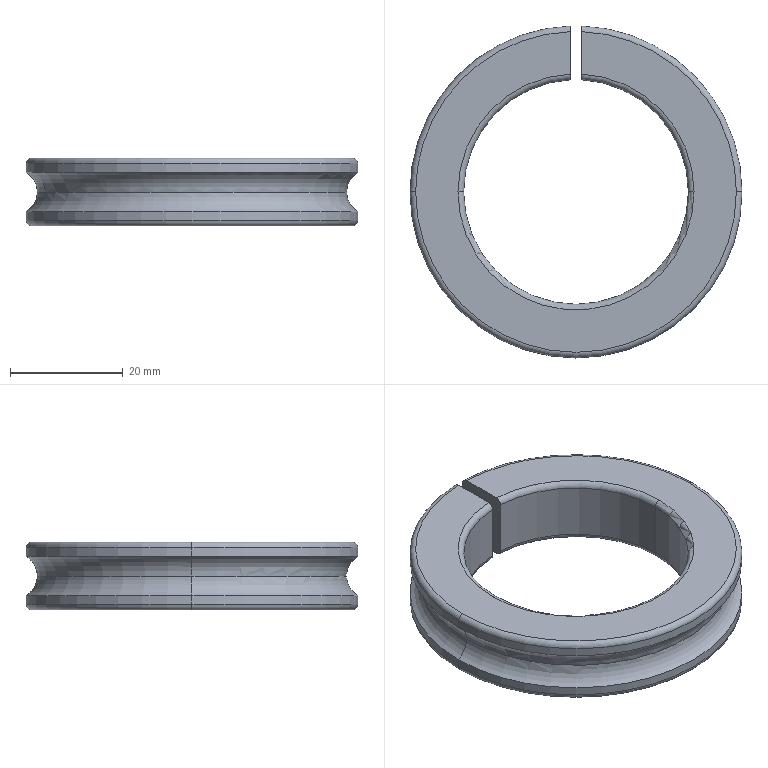Part | STEP file | 10000020578swp000-1 | 1 solid | 31 faces | box 58.8 x 58.783 x 12 mm | volume 15552 mm3 | torus 18 | cylinder 9 | plane 4 | commonest cylinder face diameters 58.8 x6 39.8 x3
STEP:
#1=CARTESIAN_POINT('',(-1.,27.382,0.));
#2=VERTEX_POINT('',#1);
#3=CARTESIAN_POINT('',(-1.,29.383,3.464));
#4=VERTEX_POINT('',#3);
#5=CARTESIAN_POINT('',(-1.,27.382,0.));
#6=CARTESIAN_POINT('',(-1.,27.382,0.1752));
#7=CARTESIAN_POINT('',(-1.,27.393,0.3515));
#8=CARTESIAN_POINT('',(-1.,27.439,0.6968));
#9=CARTESIAN_POINT('',(-1.,27.473,0.8671));
#10=CARTESIAN_POINT('',(-1.,27.608,1.371));
#11=CARTESIAN_POINT('',(-1.,27.745,1.7));
#12=CARTESIAN_POINT('',(-1.,28.005,2.151));
#13=CARTESIAN_POINT('',(-1.,28.102,2.296));
#14=CARTESIAN_POINT('',(-1.,28.315,2.573));
#15=CARTESIAN_POINT('',(-1.,28.432,2.706));
#16=CARTESIAN_POINT('',(-1.,28.802,3.076));
#17=CARTESIAN_POINT('',(-1.,29.078,3.288));
#18=CARTESIAN_POINT('',(-1.,29.383,3.464));
#19=B_SPLINE_CURVE_WITH_KNOTS('',3,(#5,#6,#7,#8,#9,#10,#11,#12,#13,#14,#15,#16,#17,#18),.UNSPECIFIED.,.F.,.F.,(4,2,2,2,2,2,4),(0.001202,0.001723,0.002244,0.003286,0.003807,0.004328,0.005371),.UNSPECIFIED.);
#20=EDGE_CURVE('',#2,#4,#19,.T.);
#21=ORIENTED_EDGE('',*,*,#20,.F.);
#22=CARTESIAN_POINT('',(-27.4,0.,0.));
#23=VERTEX_POINT('',#22);
#24=CARTESIAN_POINT('',(0.,0.,0.));
#25=DIRECTION('',(0.,0.,1.));
#26=DIRECTION('',(1.,0.,0.));
#27=AXIS2_PLACEMENT_3D('',#24,#25,#26);
#28=CIRCLE('',#27,27.4);
#29=EDGE_CURVE('',#2,#23,#28,.T.);
#30=ORIENTED_EDGE('',*,*,#29,.T.);
#31=CARTESIAN_POINT('',(-29.4,0.,3.464));
#32=VERTEX_POINT('',#31);
#33=CARTESIAN_POINT('',(-31.4,0.,0.));
#34=DIRECTION('',(0.,1.,0.));
#35=DIRECTION('',(-1.,0.,0.));
#36=AXIS2_PLACEMENT_3D('',#33,#34,#35);
#37=CIRCLE('',#36,4.);
#38=EDGE_CURVE('',#32,#23,#37,.T.);
#39=ORIENTED_EDGE('',*,*,#38,.F.);
#40=CARTESIAN_POINT('',(0.,0.,3.464));
#41=DIRECTION('',(0.,0.,-1.));
#42=DIRECTION('',(-1.,0.,0.));
#43=AXIS2_PLACEMENT_3D('',#40,#41,#42);
#44=CIRCLE('',#43,29.4);
#45=EDGE_CURVE('',#32,#4,#44,.T.);
#46=ORIENTED_EDGE('',*,*,#45,.T.);
#47=EDGE_LOOP('',(#21,#30,#39,#46));
#48=FACE_OUTER_BOUND('',#47,.T.);
#49=CARTESIAN_POINT('',(0.,0.,0.));
#50=DIRECTION('',(0.,0.,1.));
#51=DIRECTION('',(1.,0.,0.));
#52=AXIS2_PLACEMENT_3D('',#49,#50,#51);
#53=TOROIDAL_SURFACE('',#52,31.4,4.);
#54=ADVANCED_FACE('',(#48),#53,.F.);
#55=CARTESIAN_POINT('',(29.4,0.,3.464));
#56=VERTEX_POINT('',#55);
#57=CARTESIAN_POINT('',(27.4,0.,0.));
#58=VERTEX_POINT('',#57);
#59=CARTESIAN_POINT('',(31.4,0.,0.));
#60=DIRECTION('',(0.,-1.,0.));
#61=DIRECTION('',(0.,0.,-1.));
#62=AXIS2_PLACEMENT_3D('',#59,#60,#61);
#63=CIRCLE('',#62,4.);
#64=EDGE_CURVE('',#56,#58,#63,.T.);
#65=ORIENTED_EDGE('',*,*,#64,.T.);
#66=CARTESIAN_POINT('',(1.,27.382,0.));
#67=VERTEX_POINT('',#66);
#68=CARTESIAN_POINT('',(0.,0.,0.));
#69=DIRECTION('',(0.,0.,1.));
#70=DIRECTION('',(1.,0.,0.));
#71=AXIS2_PLACEMENT_3D('',#68,#69,#70);
#72=CIRCLE('',#71,27.4);
#73=EDGE_CURVE('',#58,#67,#72,.T.);
#74=ORIENTED_EDGE('',*,*,#73,.T.);
#75=CARTESIAN_POINT('',(1.,29.383,3.464));
#76=VERTEX_POINT('',#75);
#77=CARTESIAN_POINT('',(1.,29.383,3.464));
#78=CARTESIAN_POINT('',(1.,29.082,3.29));
#79=CARTESIAN_POINT('',(1.,28.799,3.073));
#80=CARTESIAN_POINT('',(1.,28.43,2.705));
#81=CARTESIAN_POINT('',(1.,28.316,2.574));
#82=CARTESIAN_POINT('',(1.,28.103,2.297));
#83=CARTESIAN_POINT('',(1.,28.004,2.15));
#84=CARTESIAN_POINT('',(1.,27.742,1.696));
#85=CARTESIAN_POINT('',(1.,27.609,1.375));
#86=CARTESIAN_POINT('',(1.,27.427,0.6953));
#87=CARTESIAN_POINT('',(1.,27.382,0.3485));
#88=CARTESIAN_POINT('',(1.,27.382,0.));
#89=B_SPLINE_CURVE_WITH_KNOTS('',3,(#77,#78,#79,#80,#81,#82,#83,#84,#85,#86,#87,#88),.UNSPECIFIED.,.F.,.F.,(4,2,2,2,2,4),(0.01965,0.02069,0.02121,0.02174,0.02278,0.02382),.UNSPECIFIED.);
#90=EDGE_CURVE('',#76,#67,#89,.T.);
#91=ORIENTED_EDGE('',*,*,#90,.F.);
#92=CARTESIAN_POINT('',(0.,0.,3.464));
#93=DIRECTION('',(0.,0.,-1.));
#94=DIRECTION('',(-1.,0.,0.));
#95=AXIS2_PLACEMENT_3D('',#92,#93,#94);
#96=CIRCLE('',#95,29.4);
#97=EDGE_CURVE('',#76,#56,#96,.T.);
#98=ORIENTED_EDGE('',*,*,#97,.T.);
#99=EDGE_LOOP('',(#65,#74,#91,#98));
#100=FACE_OUTER_BOUND('',#99,.T.);
#101=CARTESIAN_POINT('',(0.,0.,0.));
#102=DIRECTION('',(0.,0.,1.));
#103=DIRECTION('',(1.,0.,0.));
#104=AXIS2_PLACEMENT_3D('',#101,#102,#103);
#105=TOROIDAL_SURFACE('',#104,31.4,4.);
#106=ADVANCED_FACE('',(#100),#105,.F.);
#107=ORIENTED_EDGE('',*,*,#38,.T.);
#108=CARTESIAN_POINT('',(0.,0.,0.));
#109=DIRECTION('',(0.,0.,1.));
#110=DIRECTION('',(1.,0.,0.));
#111=AXIS2_PLACEMENT_3D('',#108,#109,#110);
#112=CIRCLE('',#111,27.4);
#113=EDGE_CURVE('',#23,#58,#112,.T.);
#114=ORIENTED_EDGE('',*,*,#113,.T.);
#115=ORIENTED_EDGE('',*,*,#64,.F.);
#116=CARTESIAN_POINT('',(0.,0.,3.464));
#117=DIRECTION('',(0.,0.,-1.));
#118=DIRECTION('',(-1.,0.,0.));
#119=AXIS2_PLACEMENT_3D('',#116,#117,#118);
#120=CIRCLE('',#119,29.4);
#121=EDGE_CURVE('',#56,#32,#120,.T.);
#122=ORIENTED_EDGE('',*,*,#121,.T.);
#123=EDGE_LOOP('',(#107,#114,#115,#122));
#124=FACE_OUTER_BOUND('',#123,.T.);
#125=CARTESIAN_POINT('',(0.,0.,0.));
#126=DIRECTION('',(0.,0.,1.));
#127=DIRECTION('',(1.,0.,0.));
#128=AXIS2_PLACEMENT_3D('',#125,#126,#127);
#129=TOROIDAL_SURFACE('',#128,31.4,4.);
#130=ADVANCED_FACE('',(#124),#129,.F.);
#131=CARTESIAN_POINT('',(-28.4,0.,-6.));
#132=VERTEX_POINT('',#131);
#133=CARTESIAN_POINT('',(-1.,28.382,-6.));
#134=VERTEX_POINT('',#133);
#135=CARTESIAN_POINT('',(0.,0.,-6.));
#136=DIRECTION('',(0.,0.,-1.));
#137=DIRECTION('',(1.,0.,0.));
#138=AXIS2_PLACEMENT_3D('',#135,#136,#137);
#139=CIRCLE('',#138,28.4);
#140=EDGE_CURVE('',#132,#134,#139,.T.);
#141=ORIENTED_EDGE('',*,*,#140,.F.);
#142=CARTESIAN_POINT('',(-29.4,0.,-5.));
#143=VERTEX_POINT('',#142);
#144=CARTESIAN_POINT('',(-28.4,0.,-5.));
#145=DIRECTION('',(0.,1.,0.));
#146=DIRECTION('',(-1.,0.,0.));
#147=AXIS2_PLACEMENT_3D('',#144,#145,#146);
#148=CIRCLE('',#147,1.);
#149=EDGE_CURVE('',#132,#143,#148,.T.);
#150=ORIENTED_EDGE('',*,*,#149,.T.);
#151=CARTESIAN_POINT('',(-1.,29.383,-5.));
#152=VERTEX_POINT('',#151);
#153=CARTESIAN_POINT('',(0.,0.,-5.));
#154=DIRECTION('',(0.,0.,1.));
#155=DIRECTION('',(1.,0.,0.));
#156=AXIS2_PLACEMENT_3D('',#153,#154,#155);
#157=CIRCLE('',#156,29.4);
#158=EDGE_CURVE('',#152,#143,#157,.T.);
#159=ORIENTED_EDGE('',*,*,#158,.F.);
#160=CARTESIAN_POINT('',(-1.,28.382,-6.));
#161=CARTESIAN_POINT('',(-1.,28.514,-6.));
#162=CARTESIAN_POINT('',(-1.,28.644,-5.974));
#163=CARTESIAN_POINT('',(-1.,28.886,-5.874));
#164=CARTESIAN_POINT('',(-1.,28.997,-5.8));
#165=CARTESIAN_POINT('',(-1.,29.274,-5.523));
#166=CARTESIAN_POINT('',(-1.,29.383,-5.264));
#167=CARTESIAN_POINT('',(-1.,29.383,-5.));
#168=B_SPLINE_CURVE_WITH_KNOTS('',3,(#160,#161,#162,#163,#164,#165,#166,#167),.UNSPECIFIED.,.F.,.F.,(4,2,2,4),(0.,0.0003907,0.0007813,0.001563),.UNSPECIFIED.);
#169=EDGE_CURVE('',#134,#152,#168,.T.);
#170=ORIENTED_EDGE('',*,*,#169,.F.);
#171=EDGE_LOOP('',(#141,#150,#159,#170));
#172=FACE_OUTER_BOUND('',#171,.T.);
#173=CARTESIAN_POINT('',(0.,0.,-5.));
#174=DIRECTION('',(0.,0.,1.));
#175=DIRECTION('',(1.,0.,0.));
#176=AXIS2_PLACEMENT_3D('',#173,#174,#175);
#177=TOROIDAL_SURFACE('',#176,28.4,1.);
#178=ADVANCED_FACE('',(#172),#177,.T.);
#179=ORIENTED_EDGE('',*,*,#149,.F.);
#180=CARTESIAN_POINT('',(28.4,0.,-6.));
#181=VERTEX_POINT('',#180);
#182=CARTESIAN_POINT('',(0.,0.,-6.));
#183=DIRECTION('',(0.,0.,-1.));
#184=DIRECTION('',(1.,0.,0.));
#185=AXIS2_PLACEMENT_3D('',#182,#183,#184);
#186=CIRCLE('',#185,28.4);
#187=EDGE_CURVE('',#181,#132,#186,.T.);
#188=ORIENTED_EDGE('',*,*,#187,.F.);
#189=CARTESIAN_POINT('',(29.4,0.,-5.));
#190=VERTEX_POINT('',#189);
#191=CARTESIAN_POINT('',(28.4,0.,-5.));
#192=DIRECTION('',(0.,-1.,0.));
#193=DIRECTION('',(0.,0.,-1.));
#194=AXIS2_PLACEMENT_3D('',#191,#192,#193);
#195=CIRCLE('',#194,1.);
#196=EDGE_CURVE('',#181,#190,#195,.T.);
#197=ORIENTED_EDGE('',*,*,#196,.T.);
#198=CARTESIAN_POINT('',(0.,0.,-5.));
#199=DIRECTION('',(0.,0.,1.));
#200=DIRECTION('',(1.,0.,0.));
#201=AXIS2_PLACEMENT_3D('',#198,#199,#200);
#202=CIRCLE('',#201,29.4);
#203=EDGE_CURVE('',#143,#190,#202,.T.);
#204=ORIENTED_EDGE('',*,*,#203,.F.);
#205=EDGE_LOOP('',(#179,#188,#197,#204));
#206=FACE_OUTER_BOUND('',#205,.T.);
#207=CARTESIAN_POINT('',(0.,0.,-5.));
#208=DIRECTION('',(0.,0.,1.));
#209=DIRECTION('',(1.,0.,0.));
#210=AXIS2_PLACEMENT_3D('',#207,#208,#209);
#211=TOROIDAL_SURFACE('',#210,28.4,1.);
#212=ADVANCED_FACE('',(#206),#211,.T.);
#213=CARTESIAN_POINT('',(-19.9,0.,-5.));
#214=VERTEX_POINT('',#213);
#215=CARTESIAN_POINT('',(-1.,19.875,-5.));
#216=VERTEX_POINT('',#215);
#217=CARTESIAN_POINT('',(0.,0.,-5.));
#218=DIRECTION('',(0.,0.,-1.));
#219=DIRECTION('',(1.,0.,0.));
#220=AXIS2_PLACEMENT_3D('',#217,#218,#219);
#221=CIRCLE('',#220,19.9);
#222=EDGE_CURVE('',#214,#216,#221,.T.);
#223=ORIENTED_EDGE('',*,*,#222,.F.);
#224=CARTESIAN_POINT('',(-20.9,0.,-6.));
#225=VERTEX_POINT('',#224);
#226=CARTESIAN_POINT('',(-20.9,0.,-5.));
#227=DIRECTION('',(0.,1.,0.));
#228=DIRECTION('',(-1.,0.,0.));
#229=AXIS2_PLACEMENT_3D('',#226,#227,#228);
#230=CIRCLE('',#229,1.);
#231=EDGE_CURVE('',#214,#225,#230,.T.);
#232=ORIENTED_EDGE('',*,*,#231,.T.);
#233=CARTESIAN_POINT('',(-1.,20.876,-6.));
#234=VERTEX_POINT('',#233);
#235=CARTESIAN_POINT('',(0.,0.,-6.));
#236=DIRECTION('',(0.,0.,1.));
#237=DIRECTION('',(1.,0.,0.));
#238=AXIS2_PLACEMENT_3D('',#235,#236,#237);
#239=CIRCLE('',#238,20.9);
#240=EDGE_CURVE('',#234,#225,#239,.T.);
#241=ORIENTED_EDGE('',*,*,#240,.F.);
#242=CARTESIAN_POINT('',(-1.,19.875,-5.));
#243=CARTESIAN_POINT('',(-1.,19.875,-5.132));
#244=CARTESIAN_POINT('',(-1.,19.901,-5.262));
#245=CARTESIAN_POINT('',(-1.,20.001,-5.504));
#246=CARTESIAN_POINT('',(-1.,20.076,-5.615));
#247=CARTESIAN_POINT('',(-1.,20.353,-5.891));
#248=CARTESIAN_POINT('',(-1.,20.612,-6.));
#249=CARTESIAN_POINT('',(-1.,20.876,-6.));
#250=B_SPLINE_CURVE_WITH_KNOTS('',3,(#242,#243,#244,#245,#246,#247,#248,#249),.UNSPECIFIED.,.F.,.F.,(4,2,2,4),(0.,0.0003908,0.0007815,0.001563),.UNSPECIFIED.);
#251=EDGE_CURVE('',#216,#234,#250,.T.);
#252=ORIENTED_EDGE('',*,*,#251,.F.);
#253=EDGE_LOOP('',(#223,#232,#241,#252));
#254=FACE_OUTER_BOUND('',#253,.T.);
#255=CARTESIAN_POINT('',(0.,0.,-5.));
#256=DIRECTION('',(0.,0.,1.));
#257=DIRECTION('',(1.,0.,0.));
#258=AXIS2_PLACEMENT_3D('',#255,#256,#257);
#259=TOROIDAL_SURFACE('',#258,20.9,1.);
#260=ADVANCED_FACE('',(#254),#259,.T.);
#261=ORIENTED_EDGE('',*,*,#231,.F.);
#262=CARTESIAN_POINT('',(19.9,0.,-5.));
#263=VERTEX_POINT('',#262);
#264=CARTESIAN_POINT('',(0.,0.,-5.));
#265=DIRECTION('',(0.,0.,-1.));
#266=DIRECTION('',(1.,0.,0.));
#267=AXIS2_PLACEMENT_3D('',#264,#265,#266);
#268=CIRCLE('',#267,19.9);
#269=EDGE_CURVE('',#263,#214,#268,.T.);
#270=ORIENTED_EDGE('',*,*,#269,.F.);
#271=CARTESIAN_POINT('',(20.9,0.,-6.));
#272=VERTEX_POINT('',#271);
#273=CARTESIAN_POINT('',(20.9,0.,-5.));
#274=DIRECTION('',(0.,-1.,0.));
#275=DIRECTION('',(0.,0.,-1.));
#276=AXIS2_PLACEMENT_3D('',#273,#274,#275);
#277=CIRCLE('',#276,1.);
#278=EDGE_CURVE('',#263,#272,#277,.T.);
#279=ORIENTED_EDGE('',*,*,#278,.T.);
#280=CARTESIAN_POINT('',(0.,0.,-6.));
#281=DIRECTION('',(0.,0.,1.));
#282=DIRECTION('',(1.,0.,0.));
#283=AXIS2_PLACEMENT_3D('',#280,#281,#282);
#284=CIRCLE('',#283,20.9);
#285=EDGE_CURVE('',#225,#272,#284,.T.);
#286=ORIENTED_EDGE('',*,*,#285,.F.);
#287=EDGE_LOOP('',(#261,#270,#279,#286));
#288=FACE_OUTER_BOUND('',#287,.T.);
#289=CARTESIAN_POINT('',(0.,0.,-5.));
#290=DIRECTION('',(0.,0.,1.));
#291=DIRECTION('',(1.,0.,0.));
#292=AXIS2_PLACEMENT_3D('',#289,#290,#291);
#293=TOROIDAL_SURFACE('',#292,20.9,1.);
#294=ADVANCED_FACE('',(#288),#293,.T.);
#295=CARTESIAN_POINT('',(-20.9,0.,6.));
#296=VERTEX_POINT('',#295);
#297=CARTESIAN_POINT('',(-1.,20.876,6.));
#298=VERTEX_POINT('',#297);
#299=CARTESIAN_POINT('',(0.,0.,6.));
#300=DIRECTION('',(0.,0.,-1.));
#301=DIRECTION('',(1.,0.,0.));
#302=AXIS2_PLACEMENT_3D('',#299,#300,#301);
#303=CIRCLE('',#302,20.9);
#304=EDGE_CURVE('',#296,#298,#303,.T.);
#305=ORIENTED_EDGE('',*,*,#304,.F.);
#306=CARTESIAN_POINT('',(-19.9,0.,5.));
#307=VERTEX_POINT('',#306);
#308=CARTESIAN_POINT('',(-20.9,0.,5.));
#309=DIRECTION('',(0.,1.,0.));
#310=DIRECTION('',(-1.,0.,0.));
#311=AXIS2_PLACEMENT_3D('',#308,#309,#310);
#312=CIRCLE('',#311,1.);
#313=EDGE_CURVE('',#296,#307,#312,.T.);
#314=ORIENTED_EDGE('',*,*,#313,.T.);
#315=CARTESIAN_POINT('',(-1.,19.875,5.));
#316=VERTEX_POINT('',#315);
#317=CARTESIAN_POINT('',(0.,0.,5.));
#318=DIRECTION('',(0.,0.,1.));
#319=DIRECTION('',(1.,0.,0.));
#320=AXIS2_PLACEMENT_3D('',#317,#318,#319);
#321=CIRCLE('',#320,19.9);
#322=EDGE_CURVE('',#316,#307,#321,.T.);
#323=ORIENTED_EDGE('',*,*,#322,.F.);
#324=CARTESIAN_POINT('',(-1.,20.876,6.));
#325=CARTESIAN_POINT('',(-1.,20.744,6.));
#326=CARTESIAN_POINT('',(-1.,20.614,5.974));
#327=CARTESIAN_POINT('',(-1.,20.372,5.874));
#328=CARTESIAN_POINT('',(-1.,20.261,5.8));
#329=CARTESIAN_POINT('',(-1.,19.984,5.523));
#330=CARTESIAN_POINT('',(-1.,19.875,5.264));
#331=CARTESIAN_POINT('',(-1.,19.875,5.));
#332=B_SPLINE_CURVE_WITH_KNOTS('',3,(#324,#325,#326,#327,#328,#329,#330,#331),.UNSPECIFIED.,.F.,.F.,(4,2,2,4),(0.,0.0003908,0.0007815,0.001563),.UNSPECIFIED.);
#333=EDGE_CURVE('',#298,#316,#332,.T.);
#334=ORIENTED_EDGE('',*,*,#333,.F.);
#335=EDGE_LOOP('',(#305,#314,#323,#334));
#336=FACE_OUTER_BOUND('',#335,.T.);
#337=CARTESIAN_POINT('',(0.,0.,5.));
#338=DIRECTION('',(0.,0.,1.));
#339=DIRECTION('',(1.,0.,0.));
#340=AXIS2_PLACEMENT_3D('',#337,#338,#339);
#341=TOROIDAL_SURFACE('',#340,20.9,1.);
#342=ADVANCED_FACE('',(#336),#341,.T.);
#343=ORIENTED_EDGE('',*,*,#313,.F.);
#344=CARTESIAN_POINT('',(20.9,0.,6.));
#345=VERTEX_POINT('',#344);
#346=CARTESIAN_POINT('',(0.,0.,6.));
#347=DIRECTION('',(0.,0.,-1.));
#348=DIRECTION('',(1.,0.,0.));
#349=AXIS2_PLACEMENT_3D('',#346,#347,#348);
#350=CIRCLE('',#349,20.9);
#351=EDGE_CURVE('',#345,#296,#350,.T.);
#352=ORIENTED_EDGE('',*,*,#351,.F.);
#353=CARTESIAN_POINT('',(19.9,0.,5.));
#354=VERTEX_POINT('',#353);
#355=CARTESIAN_POINT('',(20.9,0.,5.));
#356=DIRECTION('',(0.,-1.,0.));
#357=DIRECTION('',(0.,0.,-1.));
#358=AXIS2_PLACEMENT_3D('',#355,#356,#357);
#359=CIRCLE('',#358,1.);
#360=EDGE_CURVE('',#345,#354,#359,.T.);
#361=ORIENTED_EDGE('',*,*,#360,.T.);
#362=CARTESIAN_POINT('',(0.,0.,5.));
#363=DIRECTION('',(0.,0.,1.));
#364=DIRECTION('',(1.,0.,0.));
#365=AXIS2_PLACEMENT_3D('',#362,#363,#364);
#366=CIRCLE('',#365,19.9);
#367=EDGE_CURVE('',#307,#354,#366,.T.);
#368=ORIENTED_EDGE('',*,*,#367,.F.);
#369=EDGE_LOOP('',(#343,#352,#361,#368));
#370=FACE_OUTER_BOUND('',#369,.T.);
#371=CARTESIAN_POINT('',(0.,0.,5.));
#372=DIRECTION('',(0.,0.,1.));
#373=DIRECTION('',(1.,0.,0.));
#374=AXIS2_PLACEMENT_3D('',#371,#372,#373);
#375=TOROIDAL_SURFACE('',#374,20.9,1.);
#376=ADVANCED_FACE('',(#370),#375,.T.);
#377=CARTESIAN_POINT('',(-29.4,0.,5.));
#378=VERTEX_POINT('',#377);
#379=CARTESIAN_POINT('',(-1.,29.383,5.));
#380=VERTEX_POINT('',#379);
#381=CARTESIAN_POINT('',(0.,0.,5.));
#382=DIRECTION('',(0.,0.,-1.));
#383=DIRECTION('',(1.,0.,0.));
#384=AXIS2_PLACEMENT_3D('',#381,#382,#383);
#385=CIRCLE('',#384,29.4);
#386=EDGE_CURVE('',#378,#380,#385,.T.);
#387=ORIENTED_EDGE('',*,*,#386,.F.);
#388=CARTESIAN_POINT('',(-28.4,0.,6.));
#389=VERTEX_POINT('',#388);
#390=CARTESIAN_POINT('',(-28.4,0.,5.));
#391=DIRECTION('',(0.,1.,0.));
#392=DIRECTION('',(-1.,0.,0.));
#393=AXIS2_PLACEMENT_3D('',#390,#391,#392);
#394=CIRCLE('',#393,1.);
#395=EDGE_CURVE('',#378,#389,#394,.T.);
#396=ORIENTED_EDGE('',*,*,#395,.T.);
#397=CARTESIAN_POINT('',(-1.,28.382,6.));
#398=VERTEX_POINT('',#397);
#399=CARTESIAN_POINT('',(0.,0.,6.));
#400=DIRECTION('',(0.,0.,1.));
#401=DIRECTION('',(1.,0.,0.));
#402=AXIS2_PLACEMENT_3D('',#399,#400,#401);
#403=CIRCLE('',#402,28.4);
#404=EDGE_CURVE('',#398,#389,#403,.T.);
#405=ORIENTED_EDGE('',*,*,#404,.F.);
#406=CARTESIAN_POINT('',(-1.,29.383,5.));
#407=CARTESIAN_POINT('',(-1.,29.383,5.132));
#408=CARTESIAN_POINT('',(-1.,29.357,5.262));
#409=CARTESIAN_POINT('',(-1.,29.257,5.504));
#410=CARTESIAN_POINT('',(-1.,29.182,5.615));
#411=CARTESIAN_POINT('',(-1.,28.906,5.891));
#412=CARTESIAN_POINT('',(-1.,28.647,6.));
#413=CARTESIAN_POINT('',(-1.,28.382,6.));
#414=B_SPLINE_CURVE_WITH_KNOTS('',3,(#406,#407,#408,#409,#410,#411,#412,#413),.UNSPECIFIED.,.F.,.F.,(4,2,2,4),(0.,0.0003907,0.0007813,0.001563),.UNSPECIFIED.);
#415=EDGE_CURVE('',#380,#398,#414,.T.);
#416=ORIENTED_EDGE('',*,*,#415,.F.);
#417=EDGE_LOOP('',(#387,#396,#405,#416));
#418=FACE_OUTER_BOUND('',#417,.T.);
#419=CARTESIAN_POINT('',(0.,0.,5.));
#420=DIRECTION('',(0.,0.,1.));
#421=DIRECTION('',(1.,0.,0.));
#422=AXIS2_PLACEMENT_3D('',#419,#420,#421);
#423=TOROIDAL_SURFACE('',#422,28.4,1.);
#424=ADVANCED_FACE('',(#418),#423,.T.);
#425=ORIENTED_EDGE('',*,*,#395,.F.);
#426=CARTESIAN_POINT('',(29.4,0.,5.));
#427=VERTEX_POINT('',#426);
#428=CARTESIAN_POINT('',(0.,0.,5.));
#429=DIRECTION('',(0.,0.,-1.));
#430=DIRECTION('',(1.,0.,0.));
#431=AXIS2_PLACEMENT_3D('',#428,#429,#430);
#432=CIRCLE('',#431,29.4);
#433=EDGE_CURVE('',#427,#378,#432,.T.);
#434=ORIENTED_EDGE('',*,*,#433,.F.);
#435=CARTESIAN_POINT('',(28.4,0.,6.));
#436=VERTEX_POINT('',#435);
#437=CARTESIAN_POINT('',(28.4,0.,5.));
#438=DIRECTION('',(0.,-1.,0.));
#439=DIRECTION('',(0.,0.,-1.));
#440=AXIS2_PLACEMENT_3D('',#437,#438,#439);
#441=CIRCLE('',#440,1.);
#442=EDGE_CURVE('',#427,#436,#441,.T.);
#443=ORIENTED_EDGE('',*,*,#442,.T.);
#444=CARTESIAN_POINT('',(0.,0.,6.));
#445=DIRECTION('',(0.,0.,1.));
#446=DIRECTION('',(1.,0.,0.));
#447=AXIS2_PLACEMENT_3D('',#444,#445,#446);
#448=CIRCLE('',#447,28.4);
#449=EDGE_CURVE('',#389,#436,#448,.T.);
#450=ORIENTED_EDGE('',*,*,#449,.F.);
#451=EDGE_LOOP('',(#425,#434,#443,#450));
#452=FACE_OUTER_BOUND('',#451,.T.);
#453=CARTESIAN_POINT('',(0.,0.,5.));
#454=DIRECTION('',(0.,0.,1.));
#455=DIRECTION('',(1.,0.,0.));
#456=AXIS2_PLACEMENT_3D('',#453,#454,#455);
#457=TOROIDAL_SURFACE('',#456,28.4,1.);
#458=ADVANCED_FACE('',(#452),#457,.T.);
#459=ORIENTED_EDGE('',*,*,#113,.F.);
#460=CARTESIAN_POINT('',(-29.4,0.,-3.464));
#461=VERTEX_POINT('',#460);
#462=CARTESIAN_POINT('',(-31.4,0.,0.));
#463=DIRECTION('',(0.,1.,0.));
#464=DIRECTION('',(-1.,0.,0.));
#465=AXIS2_PLACEMENT_3D('',#462,#463,#464);
#466=CIRCLE('',#465,4.);
#467=EDGE_CURVE('',#23,#461,#466,.T.);
#468=ORIENTED_EDGE('',*,*,#467,.T.);
#469=CARTESIAN_POINT('',(29.4,0.,-3.464));
#470=VERTEX_POINT('',#469);
#471=CARTESIAN_POINT('',(0.,0.,-3.464));
#472=DIRECTION('',(0.,0.,1.));
#473=DIRECTION('',(1.,0.,0.));
#474=AXIS2_PLACEMENT_3D('',#471,#472,#473);
#475=CIRCLE('',#474,29.4);
#476=EDGE_CURVE('',#461,#470,#475,.T.);
#477=ORIENTED_EDGE('',*,*,#476,.T.);
#478=CARTESIAN_POINT('',(31.4,0.,0.));
#479=DIRECTION('',(0.,-1.,0.));
#480=DIRECTION('',(0.,0.,-1.));
#481=AXIS2_PLACEMENT_3D('',#478,#479,#480);
#482=CIRCLE('',#481,4.);
#483=EDGE_CURVE('',#58,#470,#482,.T.);
#484=ORIENTED_EDGE('',*,*,#483,.F.);
#485=EDGE_LOOP('',(#459,#468,#477,#484));
#486=FACE_OUTER_BOUND('',#485,.T.);
#487=CARTESIAN_POINT('',(0.,0.,0.));
#488=DIRECTION('',(0.,0.,1.));
#489=DIRECTION('',(1.,0.,0.));
#490=AXIS2_PLACEMENT_3D('',#487,#488,#489);
#491=TOROIDAL_SURFACE('',#490,31.4,4.);
#492=ADVANCED_FACE('',(#486),#491,.F.);
#493=ORIENTED_EDGE('',*,*,#73,.F.);
#494=ORIENTED_EDGE('',*,*,#483,.T.);
#495=CARTESIAN_POINT('',(1.,29.383,-3.464));
#496=VERTEX_POINT('',#495);
#497=CARTESIAN_POINT('',(0.,0.,-3.464));
#498=DIRECTION('',(0.,0.,1.));
#499=DIRECTION('',(1.,0.,0.));
#500=AXIS2_PLACEMENT_3D('',#497,#498,#499);
#501=CIRCLE('',#500,29.4);
#502=EDGE_CURVE('',#470,#496,#501,.T.);
#503=ORIENTED_EDGE('',*,*,#502,.T.);
#504=CARTESIAN_POINT('',(1.,27.382,0.));
#505=CARTESIAN_POINT('',(1.,27.382,-0.3479));
#506=CARTESIAN_POINT('',(1.,27.428,-0.6997));
#507=CARTESIAN_POINT('',(1.,27.565,-1.208));
#508=CARTESIAN_POINT('',(1.,27.621,-1.374));
#509=CARTESIAN_POINT('',(1.,27.755,-1.696));
#510=CARTESIAN_POINT('',(1.,27.832,-1.851));
#511=CARTESIAN_POINT('',(1.,28.093,-2.302));
#512=CARTESIAN_POINT('',(1.,28.309,-2.584));
#513=CARTESIAN_POINT('',(1.,28.678,-2.952));
#514=CARTESIAN_POINT('',(1.,28.808,-3.066));
#515=CARTESIAN_POINT('',(1.,29.085,-3.279));
#516=CARTESIAN_POINT('',(1.,29.232,-3.377));
#517=CARTESIAN_POINT('',(1.,29.383,-3.464));
#518=B_SPLINE_CURVE_WITH_KNOTS('',3,(#504,#505,#506,#507,#508,#509,#510,#511,#512,#513,#514,#515,#516,#517),.UNSPECIFIED.,.F.,.F.,(4,2,2,2,2,2,4),(0.02382,0.02486,0.02538,0.0259,0.02694,0.02746,0.02798),.UNSPECIFIED.);
#519=EDGE_CURVE('',#67,#496,#518,.T.);
#520=ORIENTED_EDGE('',*,*,#519,.F.);
#521=EDGE_LOOP('',(#493,#494,#503,#520));
#522=FACE_OUTER_BOUND('',#521,.T.);
#523=CARTESIAN_POINT('',(0.,0.,0.));
#524=DIRECTION('',(0.,0.,1.));
#525=DIRECTION('',(1.,0.,0.));
#526=AXIS2_PLACEMENT_3D('',#523,#524,#525);
#527=TOROIDAL_SURFACE('',#526,31.4,4.);
#528=ADVANCED_FACE('',(#522),#527,.F.);
#529=ORIENTED_EDGE('',*,*,#367,.T.);
#530=CARTESIAN_POINT('',(19.9,0.,6.));
#531=DIRECTION('',(0.,0.,-1.));
#532=VECTOR('',#531,1000.);
#533=LINE('',#530,#532);
#534=EDGE_CURVE('',#354,#263,#533,.T.);
#535=ORIENTED_EDGE('',*,*,#534,.T.);
#536=ORIENTED_EDGE('',*,*,#269,.T.);
#537=CARTESIAN_POINT('',(-19.9,0.,6.));
#538=DIRECTION('',(0.,0.,-1.));
#539=VECTOR('',#538,1000.);
#540=LINE('',#537,#539);
#541=EDGE_CURVE('',#307,#214,#540,.T.);
#542=ORIENTED_EDGE('',*,*,#541,.F.);
#543=EDGE_LOOP('',(#529,#535,#536,#542));
#544=FACE_OUTER_BOUND('',#543,.T.);
#545=CARTESIAN_POINT('',(0.,0.,6.));
#546=DIRECTION('',(0.,0.,-1.));
#547=DIRECTION('',(-1.,0.,0.));
#548=AXIS2_PLACEMENT_3D('',#545,#546,#547);
#549=CYLINDRICAL_SURFACE('',#548,19.9);
#550=ADVANCED_FACE('',(#544),#549,.F.);
#551=ORIENTED_EDGE('',*,*,#322,.T.);
#552=ORIENTED_EDGE('',*,*,#541,.T.);
#553=ORIENTED_EDGE('',*,*,#222,.T.);
#554=CARTESIAN_POINT('',(-1.,19.875,6.));
#555=DIRECTION('',(0.,0.,-1.));
#556=VECTOR('',#555,1000.);
#557=LINE('',#554,#556);
#558=EDGE_CURVE('',#316,#216,#557,.T.);
#559=ORIENTED_EDGE('',*,*,#558,.F.);
#560=EDGE_LOOP('',(#551,#552,#553,#559));
#561=FACE_OUTER_BOUND('',#560,.T.);
#562=CARTESIAN_POINT('',(0.,0.,6.));
#563=DIRECTION('',(0.,0.,-1.));
#564=DIRECTION('',(-1.,0.,0.));
#565=AXIS2_PLACEMENT_3D('',#562,#563,#564);
#566=CYLINDRICAL_SURFACE('',#565,19.9);
#567=ADVANCED_FACE('',(#561),#566,.F.);
#568=ORIENTED_EDGE('',*,*,#502,.F.);
#569=CARTESIAN_POINT('',(29.4,0.,6.));
#570=DIRECTION('',(0.,0.,-1.));
#571=VECTOR('',#570,1000.);
#572=LINE('',#569,#571);
#573=EDGE_CURVE('',#470,#190,#572,.T.);
#574=ORIENTED_EDGE('',*,*,#573,.T.);
#575=CARTESIAN_POINT('',(1.,29.383,-5.));
#576=VERTEX_POINT('',#575);
#577=CARTESIAN_POINT('',(0.,0.,-5.));
#578=DIRECTION('',(0.,0.,1.));
#579=DIRECTION('',(1.,0.,0.));
#580=AXIS2_PLACEMENT_3D('',#577,#578,#579);
#581=CIRCLE('',#580,29.4);
#582=EDGE_CURVE('',#190,#576,#581,.T.);
#583=ORIENTED_EDGE('',*,*,#582,.T.);
#584=CARTESIAN_POINT('',(1.,29.383,6.));
#585=DIRECTION('',(0.,0.,-1.));
#586=VECTOR('',#585,1000.);
#587=LINE('',#584,#586);
#588=EDGE_CURVE('',#496,#576,#587,.T.);
#589=ORIENTED_EDGE('',*,*,#588,.F.);
#590=EDGE_LOOP('',(#568,#574,#583,#589));
#591=FACE_OUTER_BOUND('',#590,.T.);
#592=CARTESIAN_POINT('',(0.,0.,6.));
#593=DIRECTION('',(0.,0.,-1.));
#594=DIRECTION('',(-1.,0.,0.));
#595=AXIS2_PLACEMENT_3D('',#592,#593,#594);
#596=CYLINDRICAL_SURFACE('',#595,29.4);
#597=ADVANCED_FACE('',(#591),#596,.T.);
#598=ORIENTED_EDGE('',*,*,#573,.F.);
#599=ORIENTED_EDGE('',*,*,#476,.F.);
#600=CARTESIAN_POINT('',(-29.4,0.,6.));
#601=DIRECTION('',(0.,0.,-1.));
#602=VECTOR('',#601,1000.);
#603=LINE('',#600,#602);
#604=EDGE_CURVE('',#461,#143,#603,.T.);
#605=ORIENTED_EDGE('',*,*,#604,.T.);
#606=ORIENTED_EDGE('',*,*,#203,.T.);
#607=EDGE_LOOP('',(#598,#599,#605,#606));
#608=FACE_OUTER_BOUND('',#607,.T.);
#609=CARTESIAN_POINT('',(0.,0.,6.));
#610=DIRECTION('',(0.,0.,-1.));
#611=DIRECTION('',(-1.,0.,0.));
#612=AXIS2_PLACEMENT_3D('',#609,#610,#611);
#613=CYLINDRICAL_SURFACE('',#612,29.4);
#614=ADVANCED_FACE('',(#608),#613,.T.);
#615=CARTESIAN_POINT('',(1.,29.383,5.));
#616=VERTEX_POINT('',#615);
#617=CARTESIAN_POINT('',(0.,0.,5.));
#618=DIRECTION('',(0.,0.,-1.));
#619=DIRECTION('',(1.,0.,0.));
#620=AXIS2_PLACEMENT_3D('',#617,#618,#619);
#621=CIRCLE('',#620,29.4);
#622=EDGE_CURVE('',#616,#427,#621,.T.);
#623=ORIENTED_EDGE('',*,*,#622,.T.);
#624=CARTESIAN_POINT('',(29.4,0.,6.));
#625=DIRECTION('',(0.,0.,-1.));
#626=VECTOR('',#625,1000.);
#627=LINE('',#624,#626);
#628=EDGE_CURVE('',#427,#56,#627,.T.);
#629=ORIENTED_EDGE('',*,*,#628,.T.);
#630=ORIENTED_EDGE('',*,*,#97,.F.);
#631=CARTESIAN_POINT('',(1.,29.383,6.));
#632=DIRECTION('',(0.,0.,-1.));
#633=VECTOR('',#632,1000.);
#634=LINE('',#631,#633);
#635=EDGE_CURVE('',#616,#76,#634,.T.);
#636=ORIENTED_EDGE('',*,*,#635,.F.);
#637=EDGE_LOOP('',(#623,#629,#630,#636));
#638=FACE_OUTER_BOUND('',#637,.T.);
#639=CARTESIAN_POINT('',(0.,0.,6.));
#640=DIRECTION('',(0.,0.,-1.));
#641=DIRECTION('',(-1.,0.,0.));
#642=AXIS2_PLACEMENT_3D('',#639,#640,#641);
#643=CYLINDRICAL_SURFACE('',#642,29.4);
#644=ADVANCED_FACE('',(#638),#643,.T.);
#645=ORIENTED_EDGE('',*,*,#628,.F.);
#646=ORIENTED_EDGE('',*,*,#433,.T.);
#647=CARTESIAN_POINT('',(-29.4,0.,6.));
#648=DIRECTION('',(0.,0.,-1.));
#649=VECTOR('',#648,1000.);
#650=LINE('',#647,#649);
#651=EDGE_CURVE('',#378,#32,#650,.T.);
#652=ORIENTED_EDGE('',*,*,#651,.T.);
#653=ORIENTED_EDGE('',*,*,#121,.F.);
#654=EDGE_LOOP('',(#645,#646,#652,#653));
#655=FACE_OUTER_BOUND('',#654,.T.);
#656=CARTESIAN_POINT('',(0.,0.,6.));
#657=DIRECTION('',(0.,0.,-1.));
#658=DIRECTION('',(-1.,0.,0.));
#659=AXIS2_PLACEMENT_3D('',#656,#657,#658);
#660=CYLINDRICAL_SURFACE('',#659,29.4);
#661=ADVANCED_FACE('',(#655),#660,.T.);
#662=ORIENTED_EDGE('',*,*,#651,.F.);
#663=ORIENTED_EDGE('',*,*,#386,.T.);
#664=CARTESIAN_POINT('',(-1.,29.383,6.));
#665=DIRECTION('',(0.,0.,-1.));
#666=VECTOR('',#665,1000.);
#667=LINE('',#664,#666);
#668=EDGE_CURVE('',#380,#4,#667,.T.);
#669=ORIENTED_EDGE('',*,*,#668,.T.);
#670=ORIENTED_EDGE('',*,*,#45,.F.);
#671=EDGE_LOOP('',(#662,#663,#669,#670));
#672=FACE_OUTER_BOUND('',#671,.T.);
#673=CARTESIAN_POINT('',(0.,0.,6.));
#674=DIRECTION('',(0.,0.,-1.));
#675=DIRECTION('',(-1.,0.,0.));
#676=AXIS2_PLACEMENT_3D('',#673,#674,#675);
#677=CYLINDRICAL_SURFACE('',#676,29.4);
#678=ADVANCED_FACE('',(#672),#677,.T.);
#679=ORIENTED_EDGE('',*,*,#604,.F.);
#680=CARTESIAN_POINT('',(-1.,29.383,-3.464));
#681=VERTEX_POINT('',#680);
#682=CARTESIAN_POINT('',(0.,0.,-3.464));
#683=DIRECTION('',(0.,0.,1.));
#684=DIRECTION('',(1.,0.,0.));
#685=AXIS2_PLACEMENT_3D('',#682,#683,#684);
#686=CIRCLE('',#685,29.4);
#687=EDGE_CURVE('',#681,#461,#686,.T.);
#688=ORIENTED_EDGE('',*,*,#687,.F.);
#689=CARTESIAN_POINT('',(-1.,29.383,6.));
#690=DIRECTION('',(0.,0.,-1.));
#691=VECTOR('',#690,1000.);
#692=LINE('',#689,#691);
#693=EDGE_CURVE('',#681,#152,#692,.T.);
#694=ORIENTED_EDGE('',*,*,#693,.T.);
#695=ORIENTED_EDGE('',*,*,#158,.T.);
#696=EDGE_LOOP('',(#679,#688,#694,#695));
#697=FACE_OUTER_BOUND('',#696,.T.);
#698=CARTESIAN_POINT('',(0.,0.,6.));
#699=DIRECTION('',(0.,0.,-1.));
#700=DIRECTION('',(-1.,0.,0.));
#701=AXIS2_PLACEMENT_3D('',#698,#699,#700);
#702=CYLINDRICAL_SURFACE('',#701,29.4);
#703=ADVANCED_FACE('',(#697),#702,.T.);
#704=CARTESIAN_POINT('',(-1.,29.383,6.));
#705=DIRECTION('',(0.,1.,0.));
#706=VECTOR('',#705,1000.);
#707=LINE('',#704,#706);
#708=EDGE_CURVE('',#298,#398,#707,.T.);
#709=ORIENTED_EDGE('',*,*,#708,.T.);
#710=ORIENTED_EDGE('',*,*,#404,.T.);
#711=ORIENTED_EDGE('',*,*,#449,.T.);
#712=CARTESIAN_POINT('',(1.,28.382,6.));
#713=VERTEX_POINT('',#712);
#714=CARTESIAN_POINT('',(0.,0.,6.));
#715=DIRECTION('',(0.,0.,1.));
#716=DIRECTION('',(1.,0.,0.));
#717=AXIS2_PLACEMENT_3D('',#714,#715,#716);
#718=CIRCLE('',#717,28.4);
#719=EDGE_CURVE('',#436,#713,#718,.T.);
#720=ORIENTED_EDGE('',*,*,#719,.T.);
#721=CARTESIAN_POINT('',(1.,20.876,6.));
#722=VERTEX_POINT('',#721);
#723=CARTESIAN_POINT('',(1.,29.383,6.));
#724=DIRECTION('',(0.,-1.,0.));
#725=VECTOR('',#724,1000.);
#726=LINE('',#723,#725);
#727=EDGE_CURVE('',#713,#722,#726,.T.);
#728=ORIENTED_EDGE('',*,*,#727,.T.);
#729=CARTESIAN_POINT('',(0.,0.,6.));
#730=DIRECTION('',(0.,0.,-1.));
#731=DIRECTION('',(1.,0.,0.));
#732=AXIS2_PLACEMENT_3D('',#729,#730,#731);
#733=CIRCLE('',#732,20.9);
#734=EDGE_CURVE('',#722,#345,#733,.T.);
#735=ORIENTED_EDGE('',*,*,#734,.T.);
#736=ORIENTED_EDGE('',*,*,#351,.T.);
#737=ORIENTED_EDGE('',*,*,#304,.T.);
#738=EDGE_LOOP('',(#709,#710,#711,#720,#728,#735,#736,#737));
#739=FACE_OUTER_BOUND('',#738,.T.);
#740=CARTESIAN_POINT('',(0.,0.,6.));
#741=DIRECTION('',(0.,0.,1.));
#742=DIRECTION('',(1.,0.,0.));
#743=AXIS2_PLACEMENT_3D('',#740,#741,#742);
#744=PLANE('',#743);
#745=ADVANCED_FACE('',(#739),#744,.T.);
#746=CARTESIAN_POINT('',(-1.,29.383,-6.));
#747=DIRECTION('',(0.,1.,0.));
#748=VECTOR('',#747,1000.);
#749=LINE('',#746,#748);
#750=EDGE_CURVE('',#234,#134,#749,.T.);
#751=ORIENTED_EDGE('',*,*,#750,.F.);
#752=ORIENTED_EDGE('',*,*,#240,.T.);
#753=ORIENTED_EDGE('',*,*,#285,.T.);
#754=CARTESIAN_POINT('',(1.,20.876,-6.));
#755=VERTEX_POINT('',#754);
#756=CARTESIAN_POINT('',(0.,0.,-6.));
#757=DIRECTION('',(0.,0.,1.));
#758=DIRECTION('',(1.,0.,0.));
#759=AXIS2_PLACEMENT_3D('',#756,#757,#758);
#760=CIRCLE('',#759,20.9);
#761=EDGE_CURVE('',#272,#755,#760,.T.);
#762=ORIENTED_EDGE('',*,*,#761,.T.);
#763=CARTESIAN_POINT('',(1.,28.382,-6.));
#764=VERTEX_POINT('',#763);
#765=CARTESIAN_POINT('',(1.,29.383,-6.));
#766=DIRECTION('',(0.,-1.,0.));
#767=VECTOR('',#766,1000.);
#768=LINE('',#765,#767);
#769=EDGE_CURVE('',#764,#755,#768,.T.);
#770=ORIENTED_EDGE('',*,*,#769,.F.);
#771=CARTESIAN_POINT('',(0.,0.,-6.));
#772=DIRECTION('',(0.,0.,-1.));
#773=DIRECTION('',(1.,0.,0.));
#774=AXIS2_PLACEMENT_3D('',#771,#772,#773);
#775=CIRCLE('',#774,28.4);
#776=EDGE_CURVE('',#764,#181,#775,.T.);
#777=ORIENTED_EDGE('',*,*,#776,.T.);
#778=ORIENTED_EDGE('',*,*,#187,.T.);
#779=ORIENTED_EDGE('',*,*,#140,.T.);
#780=EDGE_LOOP('',(#751,#752,#753,#762,#770,#777,#778,#779));
#781=FACE_OUTER_BOUND('',#780,.T.);
#782=CARTESIAN_POINT('',(0.,0.,-6.));
#783=DIRECTION('',(0.,0.,1.));
#784=DIRECTION('',(1.,0.,0.));
#785=AXIS2_PLACEMENT_3D('',#782,#783,#784);
#786=PLANE('',#785);
#787=ADVANCED_FACE('',(#781),#786,.F.);
#788=ORIENTED_EDGE('',*,*,#534,.F.);
#789=CARTESIAN_POINT('',(1.,19.875,5.));
#790=VERTEX_POINT('',#789);
#791=CARTESIAN_POINT('',(0.,0.,5.));
#792=DIRECTION('',(0.,0.,1.));
#793=DIRECTION('',(1.,0.,0.));
#794=AXIS2_PLACEMENT_3D('',#791,#792,#793);
#795=CIRCLE('',#794,19.9);
#796=EDGE_CURVE('',#354,#790,#795,.T.);
#797=ORIENTED_EDGE('',*,*,#796,.T.);
#798=CARTESIAN_POINT('',(1.,19.875,-5.));
#799=VERTEX_POINT('',#798);
#800=CARTESIAN_POINT('',(1.,19.875,6.));
#801=DIRECTION('',(0.,0.,-1.));
#802=VECTOR('',#801,1000.);
#803=LINE('',#800,#802);
#804=EDGE_CURVE('',#790,#799,#803,.T.);
#805=ORIENTED_EDGE('',*,*,#804,.T.);
#806=CARTESIAN_POINT('',(0.,0.,-5.));
#807=DIRECTION('',(0.,0.,-1.));
#808=DIRECTION('',(1.,0.,0.));
#809=AXIS2_PLACEMENT_3D('',#806,#807,#808);
#810=CIRCLE('',#809,19.9);
#811=EDGE_CURVE('',#799,#263,#810,.T.);
#812=ORIENTED_EDGE('',*,*,#811,.T.);
#813=EDGE_LOOP('',(#788,#797,#805,#812));
#814=FACE_OUTER_BOUND('',#813,.T.);
#815=CARTESIAN_POINT('',(0.,0.,6.));
#816=DIRECTION('',(0.,0.,-1.));
#817=DIRECTION('',(-1.,0.,0.));
#818=AXIS2_PLACEMENT_3D('',#815,#816,#817);
#819=CYLINDRICAL_SURFACE('',#818,19.9);
#820=ADVANCED_FACE('',(#814),#819,.F.);
#821=ORIENTED_EDGE('',*,*,#29,.F.);
#822=CARTESIAN_POINT('',(-1.,29.383,-3.464));
#823=CARTESIAN_POINT('',(-1.,29.233,-3.377));
#824=CARTESIAN_POINT('',(-1.,29.088,-3.281));
#825=CARTESIAN_POINT('',(-1.,28.811,-3.069));
#826=CARTESIAN_POINT('',(-1.,28.678,-2.952));
#827=CARTESIAN_POINT('',(-1.,28.307,-2.582));
#828=CARTESIAN_POINT('',(-1.,28.096,-2.307));
#829=CARTESIAN_POINT('',(-1.,27.743,-1.698));
#830=CARTESIAN_POINT('',(-1.,27.608,-1.371));
#831=CARTESIAN_POINT('',(-1.,27.427,-0.6945));
#832=CARTESIAN_POINT('',(-1.,27.382,-0.3503));
#833=CARTESIAN_POINT('',(-1.,27.382,0.));
#834=B_SPLINE_CURVE_WITH_KNOTS('',3,(#822,#823,#824,#825,#826,#827,#828,#829,#830,#831,#832,#833),.UNSPECIFIED.,.F.,.F.,(4,2,2,2,2,4),(0.02205,0.02257,0.02309,0.02413,0.02518,0.02622),.UNSPECIFIED.);
#835=EDGE_CURVE('',#681,#2,#834,.T.);
#836=ORIENTED_EDGE('',*,*,#835,.F.);
#837=ORIENTED_EDGE('',*,*,#687,.T.);
#838=ORIENTED_EDGE('',*,*,#467,.F.);
#839=EDGE_LOOP('',(#821,#836,#837,#838));
#840=FACE_OUTER_BOUND('',#839,.T.);
#841=CARTESIAN_POINT('',(0.,0.,0.));
#842=DIRECTION('',(0.,0.,1.));
#843=DIRECTION('',(1.,0.,0.));
#844=AXIS2_PLACEMENT_3D('',#841,#842,#843);
#845=TOROIDAL_SURFACE('',#844,31.4,4.);
#846=ADVANCED_FACE('',(#840),#845,.F.);
#847=ORIENTED_EDGE('',*,*,#727,.F.);
#848=CARTESIAN_POINT('',(1.,28.382,6.));
#849=CARTESIAN_POINT('',(1.,28.514,6.));
#850=CARTESIAN_POINT('',(1.,28.644,5.974));
#851=CARTESIAN_POINT('',(1.,28.886,5.874));
#852=CARTESIAN_POINT('',(1.,28.997,5.8));
#853=CARTESIAN_POINT('',(1.,29.274,5.523));
#854=CARTESIAN_POINT('',(1.,29.383,5.264));
#855=CARTESIAN_POINT('',(1.,29.383,5.));
#856=B_SPLINE_CURVE_WITH_KNOTS('',3,(#848,#849,#850,#851,#852,#853,#854,#855),.UNSPECIFIED.,.F.,.F.,(4,2,2,4),(0.,0.0003907,0.0007813,0.001563),.UNSPECIFIED.);
#857=EDGE_CURVE('',#713,#616,#856,.T.);
#858=ORIENTED_EDGE('',*,*,#857,.T.);
#859=ORIENTED_EDGE('',*,*,#635,.T.);
#860=ORIENTED_EDGE('',*,*,#90,.T.);
#861=ORIENTED_EDGE('',*,*,#519,.T.);
#862=ORIENTED_EDGE('',*,*,#588,.T.);
#863=CARTESIAN_POINT('',(1.,29.383,-5.));
#864=CARTESIAN_POINT('',(1.,29.383,-5.132));
#865=CARTESIAN_POINT('',(1.,29.357,-5.262));
#866=CARTESIAN_POINT('',(1.,29.257,-5.504));
#867=CARTESIAN_POINT('',(1.,29.182,-5.615));
#868=CARTESIAN_POINT('',(1.,28.906,-5.891));
#869=CARTESIAN_POINT('',(1.,28.647,-6.));
#870=CARTESIAN_POINT('',(1.,28.382,-6.));
#871=B_SPLINE_CURVE_WITH_KNOTS('',3,(#863,#864,#865,#866,#867,#868,#869,#870),.UNSPECIFIED.,.F.,.F.,(4,2,2,4),(0.,0.0003907,0.0007813,0.001563),.UNSPECIFIED.);
#872=EDGE_CURVE('',#576,#764,#871,.T.);
#873=ORIENTED_EDGE('',*,*,#872,.T.);
#874=ORIENTED_EDGE('',*,*,#769,.T.);
#875=CARTESIAN_POINT('',(1.,20.876,-6.));
#876=CARTESIAN_POINT('',(1.,20.744,-6.));
#877=CARTESIAN_POINT('',(1.,20.614,-5.974));
#878=CARTESIAN_POINT('',(1.,20.372,-5.874));
#879=CARTESIAN_POINT('',(1.,20.261,-5.8));
#880=CARTESIAN_POINT('',(1.,19.984,-5.523));
#881=CARTESIAN_POINT('',(1.,19.875,-5.264));
#882=CARTESIAN_POINT('',(1.,19.875,-5.));
#883=B_SPLINE_CURVE_WITH_KNOTS('',3,(#875,#876,#877,#878,#879,#880,#881,#882),.UNSPECIFIED.,.F.,.F.,(4,2,2,4),(0.,0.0003908,0.0007815,0.001563),.UNSPECIFIED.);
#884=EDGE_CURVE('',#755,#799,#883,.T.);
#885=ORIENTED_EDGE('',*,*,#884,.T.);
#886=ORIENTED_EDGE('',*,*,#804,.F.);
#887=CARTESIAN_POINT('',(1.,19.875,5.));
#888=CARTESIAN_POINT('',(1.,19.875,5.132));
#889=CARTESIAN_POINT('',(1.,19.901,5.262));
#890=CARTESIAN_POINT('',(1.,20.001,5.504));
#891=CARTESIAN_POINT('',(1.,20.076,5.615));
#892=CARTESIAN_POINT('',(1.,20.353,5.891));
#893=CARTESIAN_POINT('',(1.,20.612,6.));
#894=CARTESIAN_POINT('',(1.,20.876,6.));
#895=B_SPLINE_CURVE_WITH_KNOTS('',3,(#887,#888,#889,#890,#891,#892,#893,#894),.UNSPECIFIED.,.F.,.F.,(4,2,2,4),(0.,0.0003908,0.0007815,0.001563),.UNSPECIFIED.);
#896=EDGE_CURVE('',#790,#722,#895,.T.);
#897=ORIENTED_EDGE('',*,*,#896,.T.);
#898=EDGE_LOOP('',(#847,#858,#859,#860,#861,#862,#873,#874,#885,#886,#897));
#899=FACE_OUTER_BOUND('',#898,.T.);
#900=CARTESIAN_POINT('',(1.,29.383,6.));
#901=DIRECTION('',(1.,0.,0.));
#902=DIRECTION('',(0.,1.,0.));
#903=AXIS2_PLACEMENT_3D('',#900,#901,#902);
#904=PLANE('',#903);
#905=ADVANCED_FACE('',(#899),#904,.F.);
#906=ORIENTED_EDGE('',*,*,#668,.F.);
#907=ORIENTED_EDGE('',*,*,#415,.T.);
#908=ORIENTED_EDGE('',*,*,#708,.F.);
#909=ORIENTED_EDGE('',*,*,#333,.T.);
#910=ORIENTED_EDGE('',*,*,#558,.T.);
#911=ORIENTED_EDGE('',*,*,#251,.T.);
#912=ORIENTED_EDGE('',*,*,#750,.T.);
#913=ORIENTED_EDGE('',*,*,#169,.T.);
#914=ORIENTED_EDGE('',*,*,#693,.F.);
#915=ORIENTED_EDGE('',*,*,#835,.T.);
#916=ORIENTED_EDGE('',*,*,#20,.T.);
#917=EDGE_LOOP('',(#906,#907,#908,#909,#910,#911,#912,#913,#914,#915,#916));
#918=FACE_OUTER_BOUND('',#917,.T.);
#919=CARTESIAN_POINT('',(-1.,29.383,6.));
#920=DIRECTION('',(-1.,0.,0.));
#921=DIRECTION('',(0.,-1.,0.));
#922=AXIS2_PLACEMENT_3D('',#919,#920,#921);
#923=PLANE('',#922);
#924=ADVANCED_FACE('',(#918),#923,.F.);
#925=ORIENTED_EDGE('',*,*,#442,.F.);
#926=ORIENTED_EDGE('',*,*,#622,.F.);
#927=ORIENTED_EDGE('',*,*,#857,.F.);
#928=ORIENTED_EDGE('',*,*,#719,.F.);
#929=EDGE_LOOP('',(#925,#926,#927,#928));
#930=FACE_OUTER_BOUND('',#929,.T.);
#931=CARTESIAN_POINT('',(0.,0.,5.));
#932=DIRECTION('',(0.,0.,1.));
#933=DIRECTION('',(1.,0.,0.));
#934=AXIS2_PLACEMENT_3D('',#931,#932,#933);
#935=TOROIDAL_SURFACE('',#934,28.4,1.);
#936=ADVANCED_FACE('',(#930),#935,.T.);
#937=ORIENTED_EDGE('',*,*,#360,.F.);
#938=ORIENTED_EDGE('',*,*,#734,.F.);
#939=ORIENTED_EDGE('',*,*,#896,.F.);
#940=ORIENTED_EDGE('',*,*,#796,.F.);
#941=EDGE_LOOP('',(#937,#938,#939,#940));
#942=FACE_OUTER_BOUND('',#941,.T.);
#943=CARTESIAN_POINT('',(0.,0.,5.));
#944=DIRECTION('',(0.,0.,1.));
#945=DIRECTION('',(1.,0.,0.));
#946=AXIS2_PLACEMENT_3D('',#943,#944,#945);
#947=TOROIDAL_SURFACE('',#946,20.9,1.);
#948=ADVANCED_FACE('',(#942),#947,.T.);
#949=ORIENTED_EDGE('',*,*,#278,.F.);
#950=ORIENTED_EDGE('',*,*,#811,.F.);
#951=ORIENTED_EDGE('',*,*,#884,.F.);
#952=ORIENTED_EDGE('',*,*,#761,.F.);
#953=EDGE_LOOP('',(#949,#950,#951,#952));
#954=FACE_OUTER_BOUND('',#953,.T.);
#955=CARTESIAN_POINT('',(0.,0.,-5.));
#956=DIRECTION('',(0.,0.,1.));
#957=DIRECTION('',(1.,0.,0.));
#958=AXIS2_PLACEMENT_3D('',#955,#956,#957);
#959=TOROIDAL_SURFACE('',#958,20.9,1.);
#960=ADVANCED_FACE('',(#954),#959,.T.);
#961=ORIENTED_EDGE('',*,*,#196,.F.);
#962=ORIENTED_EDGE('',*,*,#776,.F.);
#963=ORIENTED_EDGE('',*,*,#872,.F.);
#964=ORIENTED_EDGE('',*,*,#582,.F.);
#965=EDGE_LOOP('',(#961,#962,#963,#964));
#966=FACE_OUTER_BOUND('',#965,.T.);
#967=CARTESIAN_POINT('',(0.,0.,-5.));
#968=DIRECTION('',(0.,0.,1.));
#969=DIRECTION('',(1.,0.,0.));
#970=AXIS2_PLACEMENT_3D('',#967,#968,#969);
#971=TOROIDAL_SURFACE('',#970,28.4,1.);
#972=ADVANCED_FACE('',(#966),#971,.T.);
#973=CLOSED_SHELL('',(#54,#106,#130,#178,#212,#260,#294,#342,#376,#424,#458,#492,#528,#550,#567,#597,#614,#644,#661,#678,#703,#745,#787,#820,#846,#905,#924,#936,#948,#960,#972));
#974=MANIFOLD_SOLID_BREP('',#973);
#975=CARTESIAN_POINT('',(0.,0.,0.));
#976=DIRECTION('',(0.,0.,1.));
#977=DIRECTION('',(1.,0.,0.));
#978=AXIS2_PLACEMENT_3D('',#975,#976,#977);
#979=(LENGTH_UNIT()NAMED_UNIT(*)SI_UNIT(.MILLI.,.METRE.));
#980=UNCERTAINTY_MEASURE_WITH_UNIT(LENGTH_MEASURE(0.00001),#979,'','');
#981=(NAMED_UNIT(*)PLANE_ANGLE_UNIT()SI_UNIT($,.RADIAN.));
#982=(NAMED_UNIT(*)SI_UNIT($,.STERADIAN.)SOLID_ANGLE_UNIT());
#983=(GEOMETRIC_REPRESENTATION_CONTEXT(3)GLOBAL_UNCERTAINTY_ASSIGNED_CONTEXT((#980))GLOBAL_UNIT_ASSIGNED_CONTEXT((#979,#981,#982))REPRESENTATION_CONTEXT('',''));
#984=ADVANCED_BREP_SHAPE_REPRESENTATION('',(#974,#978),#983);